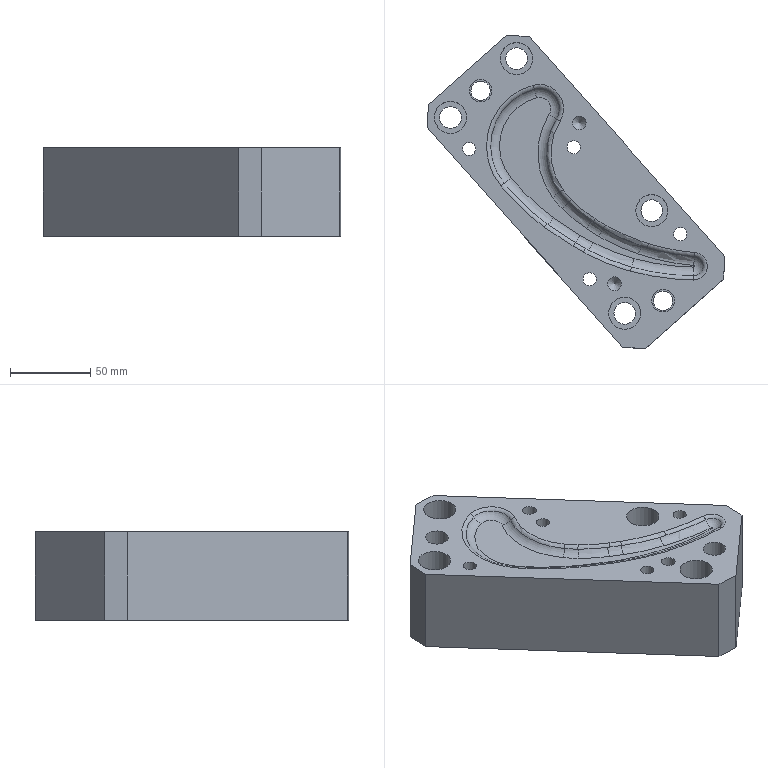Part | NX | features 23 2 | 1 solid | 73 faces | box 185.139 x 194.875 x 55 mm | volume 839032 mm3 | cylinder 22 | plane 21 | torus 16 | spline 12 | cone 2 | commonest cylinder face diameters 8.2 x4 10.31 x4 13.5 x4 20 x4 8.5 x2 12.001 x2